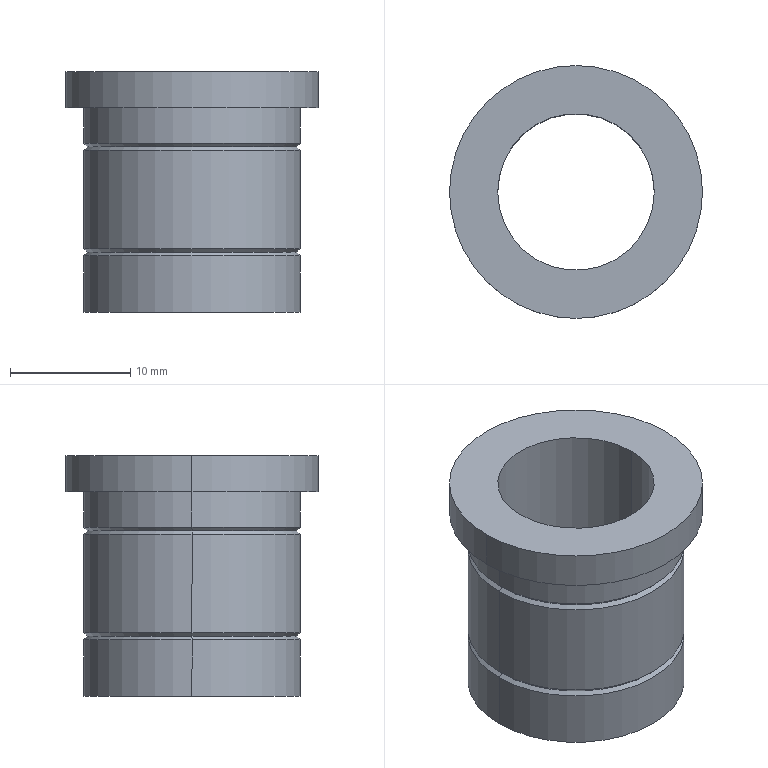Part | STEP file | SGBT13-20 | 1 solid | 21 faces | box 21 x 21 x 20 mm | volume 2700 mm3 | cylinder 10 | cone 8 | plane 3 | commonest cylinder face diameters 18 x6 13 x2 21 x2
STEP:
#1=CARTESIAN_POINT('',(6.5,0.,3.));
#2=VERTEX_POINT('',#1);
#3=CARTESIAN_POINT('',(-6.5,0.,3.));
#4=VERTEX_POINT('',#3);
#5=CARTESIAN_POINT('',(0.,0.,3.));
#6=DIRECTION('',(0.,0.,-1.));
#7=DIRECTION('',(-1.,0.,0.));
#8=AXIS2_PLACEMENT_3D('',#5,#6,#7);
#9=CIRCLE('',#8,6.5);
#10=EDGE_CURVE('',#2,#4,#9,.T.);
#11=ORIENTED_EDGE('',*,*,#10,.F.);
#12=CARTESIAN_POINT('',(6.5,0.,-17.));
#13=VERTEX_POINT('',#12);
#14=CARTESIAN_POINT('',(6.5,0.,3.));
#15=DIRECTION('',(0.,0.,-1.));
#16=VECTOR('',#15,1000.);
#17=LINE('',#14,#16);
#18=EDGE_CURVE('',#2,#13,#17,.T.);
#19=ORIENTED_EDGE('',*,*,#18,.T.);
#20=CARTESIAN_POINT('',(-6.5,0.,-17.));
#21=VERTEX_POINT('',#20);
#22=CARTESIAN_POINT('',(0.,0.,-17.));
#23=DIRECTION('',(0.,0.,1.));
#24=DIRECTION('',(-1.,0.,0.));
#25=AXIS2_PLACEMENT_3D('',#22,#23,#24);
#26=CIRCLE('',#25,6.5);
#27=EDGE_CURVE('',#21,#13,#26,.T.);
#28=ORIENTED_EDGE('',*,*,#27,.F.);
#29=CARTESIAN_POINT('',(-6.5,0.,3.));
#30=DIRECTION('',(0.,0.,-1.));
#31=VECTOR('',#30,1000.);
#32=LINE('',#29,#31);
#33=EDGE_CURVE('',#4,#21,#32,.T.);
#34=ORIENTED_EDGE('',*,*,#33,.F.);
#35=EDGE_LOOP('',(#11,#19,#28,#34));
#36=FACE_OUTER_BOUND('',#35,.T.);
#37=CARTESIAN_POINT('',(0.,0.,3.));
#38=DIRECTION('',(0.,0.,-1.));
#39=DIRECTION('',(-1.,0.,0.));
#40=AXIS2_PLACEMENT_3D('',#37,#38,#39);
#41=CYLINDRICAL_SURFACE('',#40,6.5);
#42=ADVANCED_FACE('',(#36),#41,.F.);
#43=CARTESIAN_POINT('',(-9.,0.,-17.));
#44=VERTEX_POINT('',#43);
#45=CARTESIAN_POINT('',(9.,0.,-17.));
#46=VERTEX_POINT('',#45);
#47=CARTESIAN_POINT('',(0.,0.,-17.));
#48=DIRECTION('',(0.,0.,-1.));
#49=DIRECTION('',(1.,0.,0.));
#50=AXIS2_PLACEMENT_3D('',#47,#48,#49);
#51=CIRCLE('',#50,9.);
#52=EDGE_CURVE('',#44,#46,#51,.T.);
#53=ORIENTED_EDGE('',*,*,#52,.F.);
#54=CARTESIAN_POINT('',(-9.,0.,-12.3));
#55=VERTEX_POINT('',#54);
#56=CARTESIAN_POINT('',(-9.,0.,-17.));
#57=DIRECTION('',(0.,0.,1.));
#58=VECTOR('',#57,1000.);
#59=LINE('',#56,#58);
#60=EDGE_CURVE('',#44,#55,#59,.T.);
#61=ORIENTED_EDGE('',*,*,#60,.T.);
#62=CARTESIAN_POINT('',(9.,0.,-12.3));
#63=VERTEX_POINT('',#62);
#64=CARTESIAN_POINT('',(0.,0.,-12.3));
#65=DIRECTION('',(0.,0.,-1.));
#66=DIRECTION('',(1.,0.,0.));
#67=AXIS2_PLACEMENT_3D('',#64,#65,#66);
#68=CIRCLE('',#67,9.);
#69=EDGE_CURVE('',#55,#63,#68,.T.);
#70=ORIENTED_EDGE('',*,*,#69,.T.);
#71=CARTESIAN_POINT('',(9.,0.,-17.));
#72=DIRECTION('',(0.,0.,1.));
#73=VECTOR('',#72,1000.);
#74=LINE('',#71,#73);
#75=EDGE_CURVE('',#46,#63,#74,.T.);
#76=ORIENTED_EDGE('',*,*,#75,.F.);
#77=EDGE_LOOP('',(#53,#61,#70,#76));
#78=FACE_OUTER_BOUND('',#77,.T.);
#79=CARTESIAN_POINT('',(0.,0.,-17.));
#80=DIRECTION('',(0.,0.,1.));
#81=DIRECTION('',(1.,0.,0.));
#82=AXIS2_PLACEMENT_3D('',#79,#80,#81);
#83=CYLINDRICAL_SURFACE('',#82,9.);
#84=ADVANCED_FACE('',(#78),#83,.T.);
#85=CARTESIAN_POINT('',(10.5,0.,0.));
#86=VERTEX_POINT('',#85);
#87=CARTESIAN_POINT('',(-10.5,0.,0.));
#88=VERTEX_POINT('',#87);
#89=CARTESIAN_POINT('',(0.,0.,0.));
#90=DIRECTION('',(0.,0.,1.));
#91=DIRECTION('',(1.,0.,0.));
#92=AXIS2_PLACEMENT_3D('',#89,#90,#91);
#93=CIRCLE('',#92,10.5);
#94=EDGE_CURVE('',#86,#88,#93,.T.);
#95=ORIENTED_EDGE('',*,*,#94,.T.);
#96=CARTESIAN_POINT('',(-10.5,0.,3.));
#97=VERTEX_POINT('',#96);
#98=CARTESIAN_POINT('',(-10.5,0.,0.));
#99=DIRECTION('',(0.,0.,1.));
#100=VECTOR('',#99,1000.);
#101=LINE('',#98,#100);
#102=EDGE_CURVE('',#88,#97,#101,.T.);
#103=ORIENTED_EDGE('',*,*,#102,.T.);
#104=CARTESIAN_POINT('',(10.5,0.,3.));
#105=VERTEX_POINT('',#104);
#106=CARTESIAN_POINT('',(0.,0.,3.));
#107=DIRECTION('',(0.,0.,1.));
#108=DIRECTION('',(1.,0.,0.));
#109=AXIS2_PLACEMENT_3D('',#106,#107,#108);
#110=CIRCLE('',#109,10.5);
#111=EDGE_CURVE('',#105,#97,#110,.T.);
#112=ORIENTED_EDGE('',*,*,#111,.F.);
#113=CARTESIAN_POINT('',(10.5,0.,0.));
#114=DIRECTION('',(0.,0.,1.));
#115=VECTOR('',#114,1000.);
#116=LINE('',#113,#115);
#117=EDGE_CURVE('',#86,#105,#116,.T.);
#118=ORIENTED_EDGE('',*,*,#117,.F.);
#119=EDGE_LOOP('',(#95,#103,#112,#118));
#120=FACE_OUTER_BOUND('',#119,.T.);
#121=CARTESIAN_POINT('',(0.,0.,0.));
#122=DIRECTION('',(0.,0.,1.));
#123=DIRECTION('',(1.,0.,0.));
#124=AXIS2_PLACEMENT_3D('',#121,#122,#123);
#125=CYLINDRICAL_SURFACE('',#124,10.5);
#126=ADVANCED_FACE('',(#120),#125,.T.);
#127=CARTESIAN_POINT('',(-8.7,0.,-12.));
#128=VERTEX_POINT('',#127);
#129=CARTESIAN_POINT('',(8.7,0.,-12.));
#130=VERTEX_POINT('',#129);
#131=CARTESIAN_POINT('',(0.,0.,-12.));
#132=DIRECTION('',(0.,0.,-1.));
#133=DIRECTION('',(0.,-1.,0.));
#134=AXIS2_PLACEMENT_3D('',#131,#132,#133);
#135=CIRCLE('',#134,8.7);
#136=EDGE_CURVE('',#128,#130,#135,.T.);
#137=ORIENTED_EDGE('',*,*,#136,.T.);
#138=CARTESIAN_POINT('',(9.,0.,-12.3));
#139=DIRECTION('',(0.7071,0.,-0.7071));
#140=VECTOR('',#139,1000.);
#141=LINE('',#138,#140);
#142=EDGE_CURVE('',#130,#63,#141,.T.);
#143=ORIENTED_EDGE('',*,*,#142,.T.);
#144=ORIENTED_EDGE('',*,*,#69,.F.);
#145=CARTESIAN_POINT('',(-9.,0.,-12.3));
#146=DIRECTION('',(-0.7071,0.,-0.7071));
#147=VECTOR('',#146,1000.);
#148=LINE('',#145,#147);
#149=EDGE_CURVE('',#128,#55,#148,.T.);
#150=ORIENTED_EDGE('',*,*,#149,.F.);
#151=EDGE_LOOP('',(#137,#143,#144,#150));
#152=FACE_OUTER_BOUND('',#151,.T.);
#153=CARTESIAN_POINT('',(0.,0.,-12.3));
#154=DIRECTION('',(0.,0.,-1.));
#155=DIRECTION('',(-1.,0.,0.));
#156=AXIS2_PLACEMENT_3D('',#153,#154,#155);
#157=CONICAL_SURFACE('',#156,9.,0.7854);
#158=ADVANCED_FACE('',(#152),#157,.T.);
#159=ORIENTED_EDGE('',*,*,#136,.F.);
#160=CARTESIAN_POINT('',(-9.,0.,-11.7));
#161=VERTEX_POINT('',#160);
#162=CARTESIAN_POINT('',(-9.,0.,-11.7));
#163=DIRECTION('',(-0.7071,0.,0.7071));
#164=VECTOR('',#163,1000.);
#165=LINE('',#162,#164);
#166=EDGE_CURVE('',#128,#161,#165,.T.);
#167=ORIENTED_EDGE('',*,*,#166,.T.);
#168=CARTESIAN_POINT('',(9.,0.,-11.7));
#169=VERTEX_POINT('',#168);
#170=CARTESIAN_POINT('',(0.,0.,-11.7));
#171=DIRECTION('',(0.,0.,-1.));
#172=DIRECTION('',(0.,-1.,0.));
#173=AXIS2_PLACEMENT_3D('',#170,#171,#172);
#174=CIRCLE('',#173,9.);
#175=EDGE_CURVE('',#161,#169,#174,.T.);
#176=ORIENTED_EDGE('',*,*,#175,.T.);
#177=CARTESIAN_POINT('',(9.,0.,-11.7));
#178=DIRECTION('',(0.7071,0.,0.7071));
#179=VECTOR('',#178,1000.);
#180=LINE('',#177,#179);
#181=EDGE_CURVE('',#130,#169,#180,.T.);
#182=ORIENTED_EDGE('',*,*,#181,.F.);
#183=EDGE_LOOP('',(#159,#167,#176,#182));
#184=FACE_OUTER_BOUND('',#183,.T.);
#185=CARTESIAN_POINT('',(0.,0.,-11.7));
#186=DIRECTION('',(0.,0.,1.));
#187=DIRECTION('',(1.,0.,0.));
#188=AXIS2_PLACEMENT_3D('',#185,#186,#187);
#189=CONICAL_SURFACE('',#188,9.,0.7854);
#190=ADVANCED_FACE('',(#184),#189,.T.);
#191=CARTESIAN_POINT('',(9.,0.,-2.95));
#192=VERTEX_POINT('',#191);
#193=CARTESIAN_POINT('',(-9.,0.,-2.95));
#194=VERTEX_POINT('',#193);
#195=CARTESIAN_POINT('',(0.,0.,-2.95));
#196=DIRECTION('',(0.,0.,1.));
#197=DIRECTION('',(1.,0.,0.));
#198=AXIS2_PLACEMENT_3D('',#195,#196,#197);
#199=CIRCLE('',#198,9.);
#200=EDGE_CURVE('',#192,#194,#199,.T.);
#201=ORIENTED_EDGE('',*,*,#200,.T.);
#202=CARTESIAN_POINT('',(-9.,0.,0.));
#203=VERTEX_POINT('',#202);
#204=CARTESIAN_POINT('',(-9.,0.,-2.95));
#205=DIRECTION('',(0.,0.,1.));
#206=VECTOR('',#205,1000.);
#207=LINE('',#204,#206);
#208=EDGE_CURVE('',#194,#203,#207,.T.);
#209=ORIENTED_EDGE('',*,*,#208,.T.);
#210=CARTESIAN_POINT('',(9.,0.,0.));
#211=VERTEX_POINT('',#210);
#212=CARTESIAN_POINT('',(0.,0.,0.));
#213=DIRECTION('',(0.,0.,1.));
#214=DIRECTION('',(1.,0.,0.));
#215=AXIS2_PLACEMENT_3D('',#212,#213,#214);
#216=CIRCLE('',#215,9.);
#217=EDGE_CURVE('',#211,#203,#216,.T.);
#218=ORIENTED_EDGE('',*,*,#217,.F.);
#219=CARTESIAN_POINT('',(9.,0.,-2.95));
#220=DIRECTION('',(0.,0.,1.));
#221=VECTOR('',#220,1000.);
#222=LINE('',#219,#221);
#223=EDGE_CURVE('',#192,#211,#222,.T.);
#224=ORIENTED_EDGE('',*,*,#223,.F.);
#225=EDGE_LOOP('',(#201,#209,#218,#224));
#226=FACE_OUTER_BOUND('',#225,.T.);
#227=CARTESIAN_POINT('',(0.,0.,-2.95));
#228=DIRECTION('',(0.,0.,1.));
#229=DIRECTION('',(1.,0.,0.));
#230=AXIS2_PLACEMENT_3D('',#227,#228,#229);
#231=CYLINDRICAL_SURFACE('',#230,9.);
#232=ADVANCED_FACE('',(#226),#231,.T.);
#233=ORIENTED_EDGE('',*,*,#175,.F.);
#234=CARTESIAN_POINT('',(-9.,0.,-3.55));
#235=VERTEX_POINT('',#234);
#236=CARTESIAN_POINT('',(-9.,0.,-11.7));
#237=DIRECTION('',(0.,0.,1.));
#238=VECTOR('',#237,1000.);
#239=LINE('',#236,#238);
#240=EDGE_CURVE('',#161,#235,#239,.T.);
#241=ORIENTED_EDGE('',*,*,#240,.T.);
#242=CARTESIAN_POINT('',(9.,0.,-3.55));
#243=VERTEX_POINT('',#242);
#244=CARTESIAN_POINT('',(0.,0.,-3.55));
#245=DIRECTION('',(0.,0.,-1.));
#246=DIRECTION('',(1.,0.,0.));
#247=AXIS2_PLACEMENT_3D('',#244,#245,#246);
#248=CIRCLE('',#247,9.);
#249=EDGE_CURVE('',#235,#243,#248,.T.);
#250=ORIENTED_EDGE('',*,*,#249,.T.);
#251=CARTESIAN_POINT('',(9.,0.,-11.7));
#252=DIRECTION('',(0.,0.,1.));
#253=VECTOR('',#252,1000.);
#254=LINE('',#251,#253);
#255=EDGE_CURVE('',#169,#243,#254,.T.);
#256=ORIENTED_EDGE('',*,*,#255,.F.);
#257=EDGE_LOOP('',(#233,#241,#250,#256));
#258=FACE_OUTER_BOUND('',#257,.T.);
#259=CARTESIAN_POINT('',(0.,0.,-11.7));
#260=DIRECTION('',(0.,0.,1.));
#261=DIRECTION('',(1.,0.,0.));
#262=AXIS2_PLACEMENT_3D('',#259,#260,#261);
#263=CYLINDRICAL_SURFACE('',#262,9.);
#264=ADVANCED_FACE('',(#258),#263,.T.);
#265=CARTESIAN_POINT('',(8.7,0.,-3.25));
#266=VERTEX_POINT('',#265);
#267=CARTESIAN_POINT('',(-8.7,0.,-3.25));
#268=VERTEX_POINT('',#267);
#269=CARTESIAN_POINT('',(0.,0.,-3.25));
#270=DIRECTION('',(0.,0.,1.));
#271=DIRECTION('',(0.,1.,0.));
#272=AXIS2_PLACEMENT_3D('',#269,#270,#271);
#273=CIRCLE('',#272,8.7);
#274=EDGE_CURVE('',#266,#268,#273,.T.);
#275=ORIENTED_EDGE('',*,*,#274,.T.);
#276=CARTESIAN_POINT('',(-9.,0.,-2.95));
#277=DIRECTION('',(-0.7071,0.,0.7071));
#278=VECTOR('',#277,1000.);
#279=LINE('',#276,#278);
#280=EDGE_CURVE('',#268,#194,#279,.T.);
#281=ORIENTED_EDGE('',*,*,#280,.T.);
#282=ORIENTED_EDGE('',*,*,#200,.F.);
#283=CARTESIAN_POINT('',(9.,0.,-2.95));
#284=DIRECTION('',(0.7071,0.,0.7071));
#285=VECTOR('',#284,1000.);
#286=LINE('',#283,#285);
#287=EDGE_CURVE('',#266,#192,#286,.T.);
#288=ORIENTED_EDGE('',*,*,#287,.F.);
#289=EDGE_LOOP('',(#275,#281,#282,#288));
#290=FACE_OUTER_BOUND('',#289,.T.);
#291=CARTESIAN_POINT('',(0.,0.,-2.95));
#292=DIRECTION('',(0.,0.,1.));
#293=DIRECTION('',(1.,0.,0.));
#294=AXIS2_PLACEMENT_3D('',#291,#292,#293);
#295=CONICAL_SURFACE('',#294,9.,0.7854);
#296=ADVANCED_FACE('',(#290),#295,.T.);
#297=ORIENTED_EDGE('',*,*,#274,.F.);
#298=CARTESIAN_POINT('',(9.,0.,-3.55));
#299=DIRECTION('',(0.7071,0.,-0.7071));
#300=VECTOR('',#299,1000.);
#301=LINE('',#298,#300);
#302=EDGE_CURVE('',#266,#243,#301,.T.);
#303=ORIENTED_EDGE('',*,*,#302,.T.);
#304=ORIENTED_EDGE('',*,*,#249,.F.);
#305=CARTESIAN_POINT('',(-9.,0.,-3.55));
#306=DIRECTION('',(-0.7071,0.,-0.7071));
#307=VECTOR('',#306,1000.);
#308=LINE('',#305,#307);
#309=EDGE_CURVE('',#268,#235,#308,.T.);
#310=ORIENTED_EDGE('',*,*,#309,.F.);
#311=EDGE_LOOP('',(#297,#303,#304,#310));
#312=FACE_OUTER_BOUND('',#311,.T.);
#313=CARTESIAN_POINT('',(0.,0.,-3.55));
#314=DIRECTION('',(0.,0.,-1.));
#315=DIRECTION('',(-1.,0.,0.));
#316=AXIS2_PLACEMENT_3D('',#313,#314,#315);
#317=CONICAL_SURFACE('',#316,9.,0.7854);
#318=ADVANCED_FACE('',(#312),#317,.T.);
#319=ORIENTED_EDGE('',*,*,#18,.F.);
#320=CARTESIAN_POINT('',(0.,0.,3.));
#321=DIRECTION('',(0.,0.,-1.));
#322=DIRECTION('',(-1.,0.,0.));
#323=AXIS2_PLACEMENT_3D('',#320,#321,#322);
#324=CIRCLE('',#323,6.5);
#325=EDGE_CURVE('',#4,#2,#324,.T.);
#326=ORIENTED_EDGE('',*,*,#325,.F.);
#327=ORIENTED_EDGE('',*,*,#33,.T.);
#328=CARTESIAN_POINT('',(0.,0.,-17.));
#329=DIRECTION('',(0.,0.,1.));
#330=DIRECTION('',(-1.,0.,0.));
#331=AXIS2_PLACEMENT_3D('',#328,#329,#330);
#332=CIRCLE('',#331,6.5);
#333=EDGE_CURVE('',#13,#21,#332,.T.);
#334=ORIENTED_EDGE('',*,*,#333,.F.);
#335=EDGE_LOOP('',(#319,#326,#327,#334));
#336=FACE_OUTER_BOUND('',#335,.T.);
#337=CARTESIAN_POINT('',(0.,0.,3.));
#338=DIRECTION('',(0.,0.,-1.));
#339=DIRECTION('',(-1.,0.,0.));
#340=AXIS2_PLACEMENT_3D('',#337,#338,#339);
#341=CYLINDRICAL_SURFACE('',#340,6.5);
#342=ADVANCED_FACE('',(#336),#341,.F.);
#343=ORIENTED_EDGE('',*,*,#27,.T.);
#344=ORIENTED_EDGE('',*,*,#333,.T.);
#345=EDGE_LOOP('',(#343,#344));
#346=FACE_BOUND('',#345,.T.);
#347=CARTESIAN_POINT('',(0.,0.,-17.));
#348=DIRECTION('',(0.,0.,-1.));
#349=DIRECTION('',(1.,0.,0.));
#350=AXIS2_PLACEMENT_3D('',#347,#348,#349);
#351=CIRCLE('',#350,9.);
#352=EDGE_CURVE('',#46,#44,#351,.T.);
#353=ORIENTED_EDGE('',*,*,#352,.T.);
#354=ORIENTED_EDGE('',*,*,#52,.T.);
#355=EDGE_LOOP('',(#353,#354));
#356=FACE_OUTER_BOUND('',#355,.T.);
#357=CARTESIAN_POINT('',(0.,0.,-17.));
#358=DIRECTION('',(0.,0.,-1.));
#359=DIRECTION('',(-1.,0.,0.));
#360=AXIS2_PLACEMENT_3D('',#357,#358,#359);
#361=PLANE('',#360);
#362=ADVANCED_FACE('',(#346,#356),#361,.T.);
#363=ORIENTED_EDGE('',*,*,#325,.T.);
#364=ORIENTED_EDGE('',*,*,#10,.T.);
#365=EDGE_LOOP('',(#363,#364));
#366=FACE_BOUND('',#365,.T.);
#367=ORIENTED_EDGE('',*,*,#111,.T.);
#368=CARTESIAN_POINT('',(0.,0.,3.));
#369=DIRECTION('',(0.,0.,1.));
#370=DIRECTION('',(1.,0.,0.));
#371=AXIS2_PLACEMENT_3D('',#368,#369,#370);
#372=CIRCLE('',#371,10.5);
#373=EDGE_CURVE('',#97,#105,#372,.T.);
#374=ORIENTED_EDGE('',*,*,#373,.T.);
#375=EDGE_LOOP('',(#367,#374));
#376=FACE_OUTER_BOUND('',#375,.T.);
#377=CARTESIAN_POINT('',(0.,0.,3.));
#378=DIRECTION('',(0.,0.,1.));
#379=DIRECTION('',(1.,0.,0.));
#380=AXIS2_PLACEMENT_3D('',#377,#378,#379);
#381=PLANE('',#380);
#382=ADVANCED_FACE('',(#366,#376),#381,.T.);
#383=ORIENTED_EDGE('',*,*,#60,.F.);
#384=ORIENTED_EDGE('',*,*,#352,.F.);
#385=ORIENTED_EDGE('',*,*,#75,.T.);
#386=CARTESIAN_POINT('',(0.,0.,-12.3));
#387=DIRECTION('',(0.,0.,-1.));
#388=DIRECTION('',(1.,0.,0.));
#389=AXIS2_PLACEMENT_3D('',#386,#387,#388);
#390=CIRCLE('',#389,9.);
#391=EDGE_CURVE('',#63,#55,#390,.T.);
#392=ORIENTED_EDGE('',*,*,#391,.T.);
#393=EDGE_LOOP('',(#383,#384,#385,#392));
#394=FACE_OUTER_BOUND('',#393,.T.);
#395=CARTESIAN_POINT('',(0.,0.,-17.));
#396=DIRECTION('',(0.,0.,1.));
#397=DIRECTION('',(1.,0.,0.));
#398=AXIS2_PLACEMENT_3D('',#395,#396,#397);
#399=CYLINDRICAL_SURFACE('',#398,9.);
#400=ADVANCED_FACE('',(#394),#399,.T.);
#401=ORIENTED_EDGE('',*,*,#102,.F.);
#402=CARTESIAN_POINT('',(0.,0.,0.));
#403=DIRECTION('',(0.,0.,1.));
#404=DIRECTION('',(1.,0.,0.));
#405=AXIS2_PLACEMENT_3D('',#402,#403,#404);
#406=CIRCLE('',#405,10.5);
#407=EDGE_CURVE('',#88,#86,#406,.T.);
#408=ORIENTED_EDGE('',*,*,#407,.T.);
#409=ORIENTED_EDGE('',*,*,#117,.T.);
#410=ORIENTED_EDGE('',*,*,#373,.F.);
#411=EDGE_LOOP('',(#401,#408,#409,#410));
#412=FACE_OUTER_BOUND('',#411,.T.);
#413=CARTESIAN_POINT('',(0.,0.,0.));
#414=DIRECTION('',(0.,0.,1.));
#415=DIRECTION('',(1.,0.,0.));
#416=AXIS2_PLACEMENT_3D('',#413,#414,#415);
#417=CYLINDRICAL_SURFACE('',#416,10.5);
#418=ADVANCED_FACE('',(#412),#417,.T.);
#419=ORIENTED_EDGE('',*,*,#142,.F.);
#420=CARTESIAN_POINT('',(0.,0.,-12.));
#421=DIRECTION('',(0.,0.,-1.));
#422=DIRECTION('',(0.,-1.,0.));
#423=AXIS2_PLACEMENT_3D('',#420,#421,#422);
#424=CIRCLE('',#423,8.7);
#425=EDGE_CURVE('',#130,#128,#424,.T.);
#426=ORIENTED_EDGE('',*,*,#425,.T.);
#427=ORIENTED_EDGE('',*,*,#149,.T.);
#428=ORIENTED_EDGE('',*,*,#391,.F.);
#429=EDGE_LOOP('',(#419,#426,#427,#428));
#430=FACE_OUTER_BOUND('',#429,.T.);
#431=CARTESIAN_POINT('',(0.,0.,-12.3));
#432=DIRECTION('',(0.,0.,-1.));
#433=DIRECTION('',(-1.,0.,0.));
#434=AXIS2_PLACEMENT_3D('',#431,#432,#433);
#435=CONICAL_SURFACE('',#434,9.,0.7854);
#436=ADVANCED_FACE('',(#430),#435,.T.);
#437=ORIENTED_EDGE('',*,*,#217,.T.);
#438=CARTESIAN_POINT('',(0.,0.,0.));
#439=DIRECTION('',(0.,0.,1.));
#440=DIRECTION('',(1.,0.,0.));
#441=AXIS2_PLACEMENT_3D('',#438,#439,#440);
#442=CIRCLE('',#441,9.);
#443=EDGE_CURVE('',#203,#211,#442,.T.);
#444=ORIENTED_EDGE('',*,*,#443,.T.);
#445=EDGE_LOOP('',(#437,#444));
#446=FACE_BOUND('',#445,.T.);
#447=ORIENTED_EDGE('',*,*,#94,.F.);
#448=ORIENTED_EDGE('',*,*,#407,.F.);
#449=EDGE_LOOP('',(#447,#448));
#450=FACE_OUTER_BOUND('',#449,.T.);
#451=CARTESIAN_POINT('',(0.,0.,0.));
#452=DIRECTION('',(0.,0.,-1.));
#453=DIRECTION('',(-1.,0.,0.));
#454=AXIS2_PLACEMENT_3D('',#451,#452,#453);
#455=PLANE('',#454);
#456=ADVANCED_FACE('',(#446,#450),#455,.T.);
#457=ORIENTED_EDGE('',*,*,#166,.F.);
#458=ORIENTED_EDGE('',*,*,#425,.F.);
#459=ORIENTED_EDGE('',*,*,#181,.T.);
#460=CARTESIAN_POINT('',(0.,0.,-11.7));
#461=DIRECTION('',(0.,0.,-1.));
#462=DIRECTION('',(0.,-1.,0.));
#463=AXIS2_PLACEMENT_3D('',#460,#461,#462);
#464=CIRCLE('',#463,9.);
#465=EDGE_CURVE('',#169,#161,#464,.T.);
#466=ORIENTED_EDGE('',*,*,#465,.T.);
#467=EDGE_LOOP('',(#457,#458,#459,#466));
#468=FACE_OUTER_BOUND('',#467,.T.);
#469=CARTESIAN_POINT('',(0.,0.,-11.7));
#470=DIRECTION('',(0.,0.,1.));
#471=DIRECTION('',(1.,0.,0.));
#472=AXIS2_PLACEMENT_3D('',#469,#470,#471);
#473=CONICAL_SURFACE('',#472,9.,0.7854);
#474=ADVANCED_FACE('',(#468),#473,.T.);
#475=ORIENTED_EDGE('',*,*,#208,.F.);
#476=CARTESIAN_POINT('',(0.,0.,-2.95));
#477=DIRECTION('',(0.,0.,1.));
#478=DIRECTION('',(1.,0.,0.));
#479=AXIS2_PLACEMENT_3D('',#476,#477,#478);
#480=CIRCLE('',#479,9.);
#481=EDGE_CURVE('',#194,#192,#480,.T.);
#482=ORIENTED_EDGE('',*,*,#481,.T.);
#483=ORIENTED_EDGE('',*,*,#223,.T.);
#484=ORIENTED_EDGE('',*,*,#443,.F.);
#485=EDGE_LOOP('',(#475,#482,#483,#484));
#486=FACE_OUTER_BOUND('',#485,.T.);
#487=CARTESIAN_POINT('',(0.,0.,-2.95));
#488=DIRECTION('',(0.,0.,1.));
#489=DIRECTION('',(1.,0.,0.));
#490=AXIS2_PLACEMENT_3D('',#487,#488,#489);
#491=CYLINDRICAL_SURFACE('',#490,9.);
#492=ADVANCED_FACE('',(#486),#491,.T.);
#493=ORIENTED_EDGE('',*,*,#240,.F.);
#494=ORIENTED_EDGE('',*,*,#465,.F.);
#495=ORIENTED_EDGE('',*,*,#255,.T.);
#496=CARTESIAN_POINT('',(0.,0.,-3.55));
#497=DIRECTION('',(0.,0.,-1.));
#498=DIRECTION('',(1.,0.,0.));
#499=AXIS2_PLACEMENT_3D('',#496,#497,#498);
#500=CIRCLE('',#499,9.);
#501=EDGE_CURVE('',#243,#235,#500,.T.);
#502=ORIENTED_EDGE('',*,*,#501,.T.);
#503=EDGE_LOOP('',(#493,#494,#495,#502));
#504=FACE_OUTER_BOUND('',#503,.T.);
#505=CARTESIAN_POINT('',(0.,0.,-11.7));
#506=DIRECTION('',(0.,0.,1.));
#507=DIRECTION('',(1.,0.,0.));
#508=AXIS2_PLACEMENT_3D('',#505,#506,#507);
#509=CYLINDRICAL_SURFACE('',#508,9.);
#510=ADVANCED_FACE('',(#504),#509,.T.);
#511=ORIENTED_EDGE('',*,*,#280,.F.);
#512=CARTESIAN_POINT('',(0.,0.,-3.25));
#513=DIRECTION('',(0.,0.,1.));
#514=DIRECTION('',(0.,1.,0.));
#515=AXIS2_PLACEMENT_3D('',#512,#513,#514);
#516=CIRCLE('',#515,8.7);
#517=EDGE_CURVE('',#268,#266,#516,.T.);
#518=ORIENTED_EDGE('',*,*,#517,.T.);
#519=ORIENTED_EDGE('',*,*,#287,.T.);
#520=ORIENTED_EDGE('',*,*,#481,.F.);
#521=EDGE_LOOP('',(#511,#518,#519,#520));
#522=FACE_OUTER_BOUND('',#521,.T.);
#523=CARTESIAN_POINT('',(0.,0.,-2.95));
#524=DIRECTION('',(0.,0.,1.));
#525=DIRECTION('',(1.,0.,0.));
#526=AXIS2_PLACEMENT_3D('',#523,#524,#525);
#527=CONICAL_SURFACE('',#526,9.,0.7854);
#528=ADVANCED_FACE('',(#522),#527,.T.);
#529=ORIENTED_EDGE('',*,*,#302,.F.);
#530=ORIENTED_EDGE('',*,*,#517,.F.);
#531=ORIENTED_EDGE('',*,*,#309,.T.);
#532=ORIENTED_EDGE('',*,*,#501,.F.);
#533=EDGE_LOOP('',(#529,#530,#531,#532));
#534=FACE_OUTER_BOUND('',#533,.T.);
#535=CARTESIAN_POINT('',(0.,0.,-3.55));
#536=DIRECTION('',(0.,0.,-1.));
#537=DIRECTION('',(-1.,0.,0.));
#538=AXIS2_PLACEMENT_3D('',#535,#536,#537);
#539=CONICAL_SURFACE('',#538,9.,0.7854);
#540=ADVANCED_FACE('',(#534),#539,.T.);
#541=CLOSED_SHELL('',(#42,#84,#126,#158,#190,#232,#264,#296,#318,#342,#362,#382,#400,#418,#436,#456,#474,#492,#510,#528,#540));
#542=MANIFOLD_SOLID_BREP('',#541);
#543=CARTESIAN_POINT('',(0.,0.,0.));
#544=DIRECTION('',(0.,0.,1.));
#545=DIRECTION('',(1.,0.,0.));
#546=AXIS2_PLACEMENT_3D('',#543,#544,#545);
#547=(LENGTH_UNIT()NAMED_UNIT(*)SI_UNIT(.MILLI.,.METRE.));
#548=UNCERTAINTY_MEASURE_WITH_UNIT(LENGTH_MEASURE(0.00001),#547,'','');
#549=(NAMED_UNIT(*)PLANE_ANGLE_UNIT()SI_UNIT($,.RADIAN.));
#550=(NAMED_UNIT(*)SI_UNIT($,.STERADIAN.)SOLID_ANGLE_UNIT());
#551=(GEOMETRIC_REPRESENTATION_CONTEXT(3)GLOBAL_UNCERTAINTY_ASSIGNED_CONTEXT((#548))GLOBAL_UNIT_ASSIGNED_CONTEXT((#547,#549,#550))REPRESENTATION_CONTEXT('',''));
#552=ADVANCED_BREP_SHAPE_REPRESENTATION('',(#542,#546),#551);